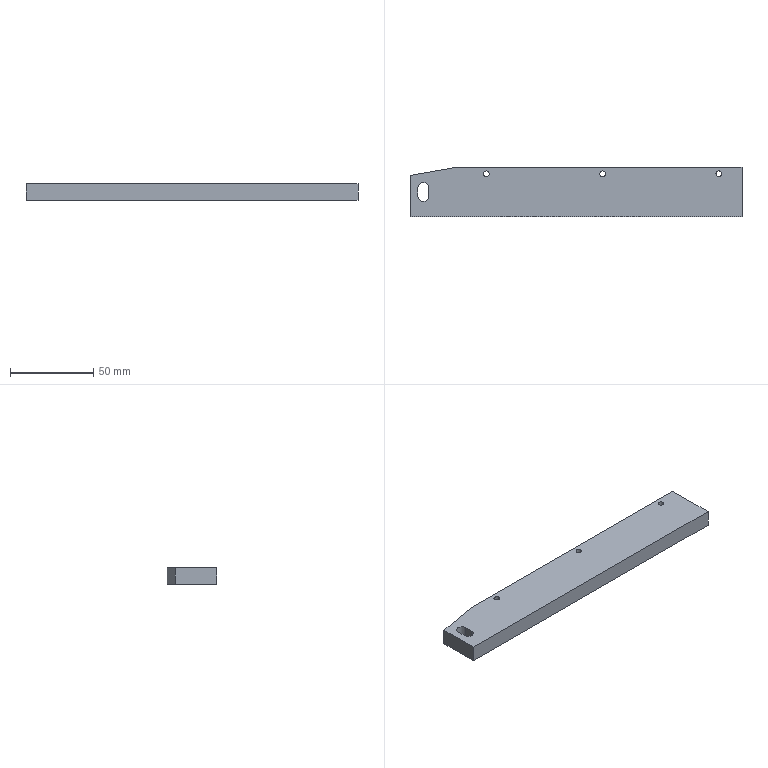Part | STEP file | CA-10-006Lift Stop Plate2_Default | 1 solid | 26 faces | box 200 x 30 x 10 mm | volume 58212 mm3 | cylinder 14 | plane 12 | commonest cylinder face diameters 3.4 x6 5.5 x6 6.5 x2